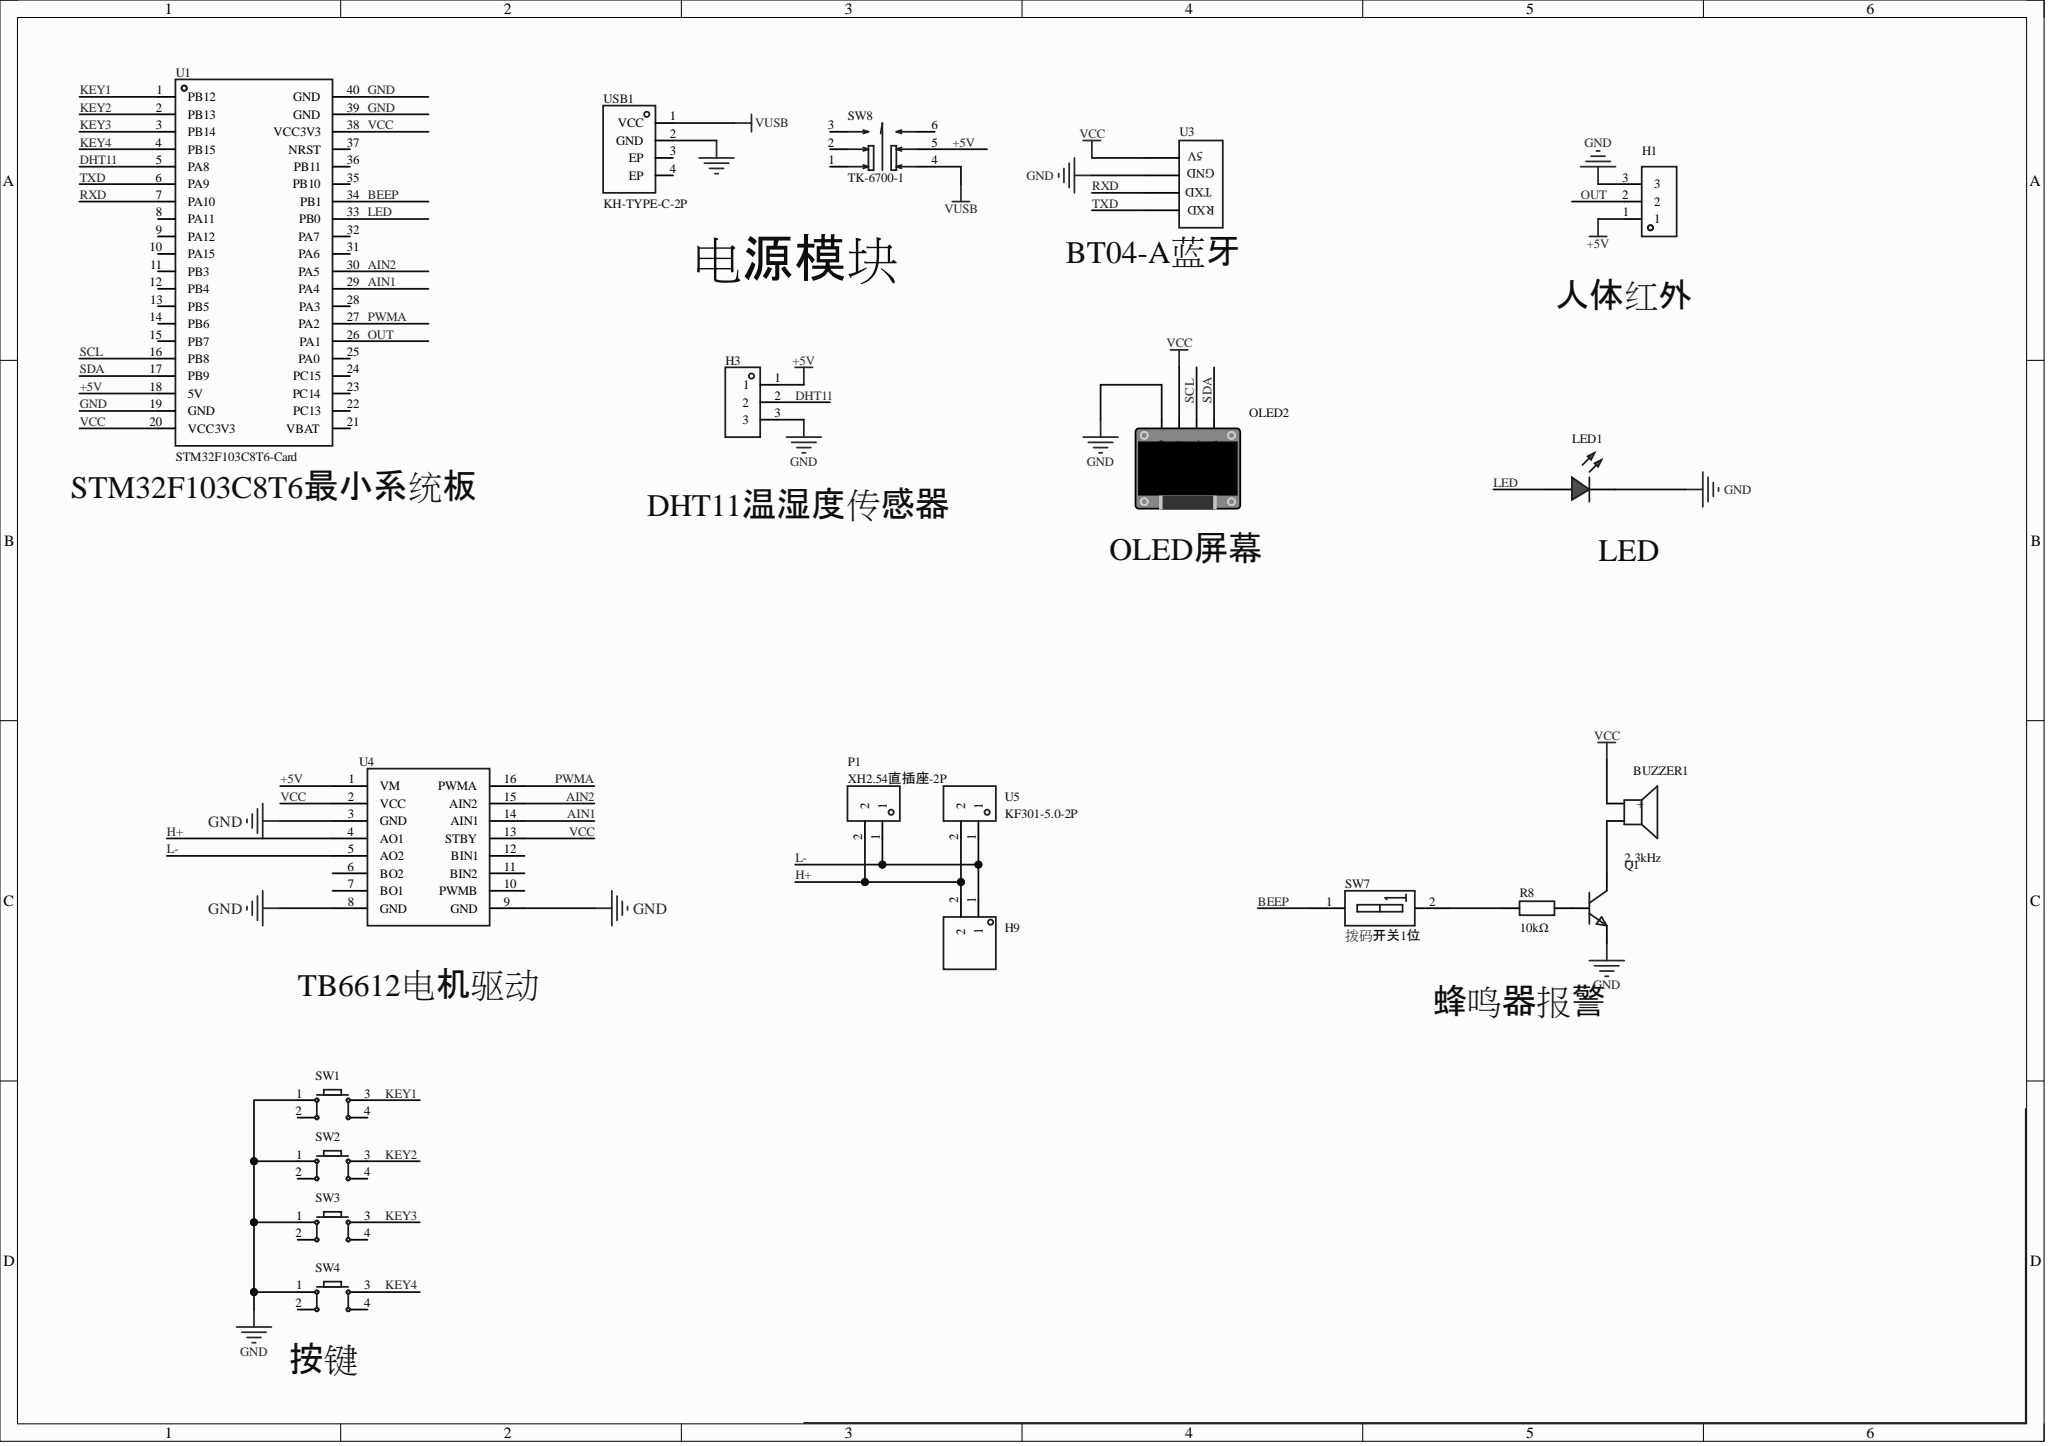Circuit board | Altium Designer | 20 parts | 24 nets
Bill of materials:
Comment,Description,Designator,Footprint,LibRef,Quantity
"2.3kHz","","BUZZER1","BUZ-TH_BD12.0-P7.60-D0.6-FD","TMB12A05_C96093","1"
"","","H1, H3","HDR-TH_3P-P2.54-V-F","HDR-F_2.54_1x3P","2"
"","","H9","HDR-TH_2P-P2.54-V-M-1","HDR-M_2.54_1x2P","1"
"","","LED1","LED_TH-3mm","LED_TH-R_3mm","1"
"","","OLED2","0.96OLED_4P","0.96OLED模块_4P","1"
"XH2.54直插座-2P","","P1","CONN-TH_XH2.54-2P","XH2.54直插座-2P","1"
"","","Q1","S8050_TO_92","S8050_TO_NPN","1"
"10kΩ","","R8","Res_1/4W","Res_AXIAL-1/4W","1"
"","","SW1, SW2, SW3, SW4","SW-TH_4P-L6.0-W6.0-P4.50-LS6.5","Key_TH_6x6x6","4"
"拨码开关1位","","SW7","SW-TH_2P-L3.9-W9.9-P2.54-LS7.6","NDS-01V_C501305","1"
"TK-6700-1","","SW8","SW-TH_TK-6700-1","TK-6700-1","1"
"STM32F103C8T6-Card","","U1","CONN-TH_L53.3-W22.9_STM32F103C8T6-CARD","STM32F103C8T6-Card","1"
"","","U3","BT04-A","bt04","1"
"","","U4","tb6612","tb6612","1"
"KF301-5.0-2P","","U5","CONN-TH_P5.00_KF301-5.0-2P","KF301-5.0-2P","1"
"KH-TYPE-C-2P","","USB1","USB-SMD_KH-TYPE-C-2P","KH-TYPE-C-2P","1"
Netlist (Protel format):
[
BUZZER1
BUZ-TH_BD12.0-P7.60-D0.6-FD
2.3kHz



]
[
H1
HDR-TH_3P-P2.54-V-F




]
[
H3
HDR-TH_3P-P2.54-V-F




]
[
H9
HDR-TH_2P-P2.54-V-M-1




]
[
LED1
LED_TH-3mm




]
[
OLED2
0.96OLED_4P




]
[
P1
CONN-TH_XH2.54-2P
XH2.54直插座-2P



]
[
Q1
S8050_TO_92




]
[
R8
Res_1/4W
10kΩ



]
[
SW1
SW-TH_4P-L6.0-W6.0-P4.50-LS6.5




]
[
SW2
SW-TH_4P-L6.0-W6.0-P4.50-LS6.5




]
[
SW3
SW-TH_4P-L6.0-W6.0-P4.50-LS6.5




]
[
SW4
SW-TH_4P-L6.0-W6.0-P4.50-LS6.5




]
[
SW7
SW-TH_2P-L3.9-W9.9-P2.54-LS7.6
拨码开关1位



]
[
SW8
SW-TH_TK-6700-1
TK-6700-1



]
[
U1
CONN-TH_L53.3-W22.9_STM32F103C8T6-CARD
STM32F103C8T6-Card



]
[
U3
BT04-A




]
[
U4
tb6612




]
[
U5
CONN-TH_P5.00_KF301-5.0-2P
KF301-5.0-2P



]
[
USB1
USB-SMD_KH-TYPE-C-2P
KH-TYPE-C-2P



]
(
VUSB
SW8-4
USB1-1
)
(
VCC
BUZZER1-1
OLED2-2
U1-20
U1-38
U3-4
U4-2
U4-13
)
(
TXD
U1-6
U3-1
)
(
SDA
OLED2-4
U1-17
)
(
SCL
OLED2-3
U1-16
)
(
RXD
U1-7
U3-2
)
(
PWMA
U1-27
U4-16
)
(
OUT
H1-2
U1-26
)
(
NetR8_1
R8-1
SW7-2
)
(
NetQ1_2
Q1-2
R8-2
)
(
NetBUZZER1_2
BUZZER1-2
Q1-3
)
(
LED
LED1-1
U1-33
)
(
L-
H9-1
P1-1
U4-5
U5-1
)
(
KEY4
SW4-3
U1-4
)
(
KEY3
SW3-3
U1-3
)
(
KEY2
SW2-3
U1-2
)
(
KEY1
SW1-3
U1-1
)
(
H+
H9-2
P1-2
U4-4
U5-2
)
(
GND
H1-3
H3-3
LED1-2
OLED2-1
Q1-1
SW1-1
SW2-1
SW3-1
SW4-1
U1-19
U1-39
U1-40
U3-3
U4-3
U4-8
U4-9
USB1-2
)
(
DHT11
H3-2
U1-5
)
(
BEEP
SW7-1
U1-34
)
(
AIN2
U1-30
U4-15
)
(
AIN1
U1-29
U4-14
)
(
+5V
H1-1
H3-1
SW8-5
U1-18
U4-1
)